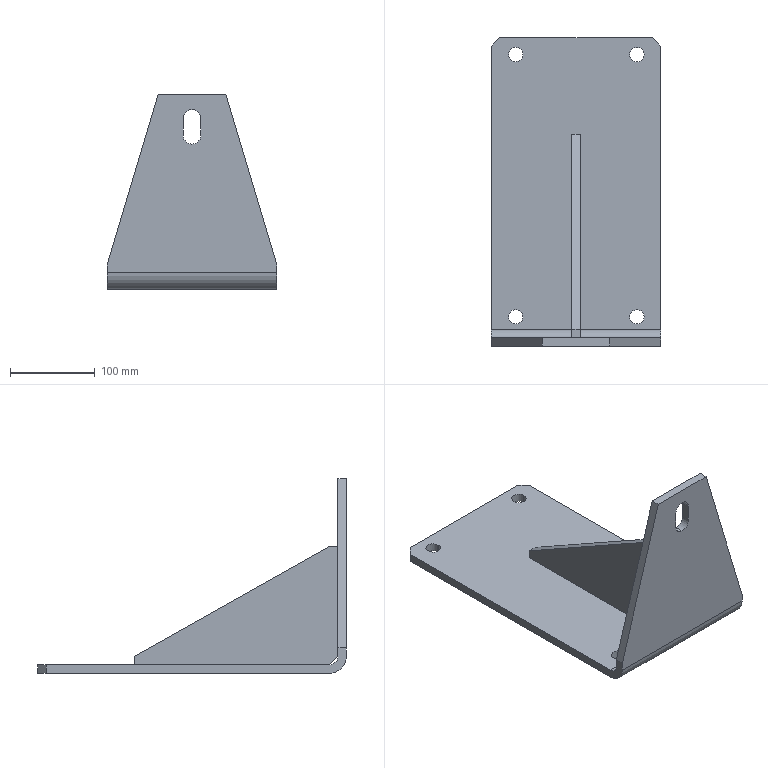Part | SolidWorks | features Chamfer 1, MBimport 1 | 1 solid | 33 faces | box 200 x 365 x 230 mm | volume 1205759 mm3 | plane 20 | cylinder 13 | commonest cylinder face diameters 17 x8 21 x3 20 x1 40 x1
STEP:
#1=CARTESIAN_POINT('',(183.597,184.249,10.));
#2=VERTEX_POINT('',#1);
#3=CARTESIAN_POINT('',(193.597,184.249,10.));
#4=VERTEX_POINT('',#3);
#5=CARTESIAN_POINT('',(183.597,184.249,10.));
#6=DIRECTION('',(1.,0.,0.));
#7=VECTOR('',#6,1000.);
#8=LINE('',#5,#7);
#9=EDGE_CURVE('',#2,#4,#8,.T.);
#10=ORIENTED_EDGE('',*,*,#9,.F.);
#11=CARTESIAN_POINT('',(88.597,184.249,10.));
#12=VERTEX_POINT('',#11);
#13=CARTESIAN_POINT('',(288.597,184.249,10.));
#14=DIRECTION('',(1.,0.,0.));
#15=VECTOR('',#14,1000.);
#16=LINE('',#13,#15);
#17=EDGE_CURVE('',#12,#2,#16,.T.);
#18=ORIENTED_EDGE('',*,*,#17,.F.);
#19=CARTESIAN_POINT('',(88.597,174.249,20.));
#20=VERTEX_POINT('',#19);
#21=CARTESIAN_POINT('',(88.597,184.249,20.));
#22=DIRECTION('',(1.,0.,0.));
#23=DIRECTION('',(0.,1.,0.));
#24=AXIS2_PLACEMENT_3D('',#21,#22,#23);
#25=CIRCLE('',#24,10.);
#26=EDGE_CURVE('',#20,#12,#25,.T.);
#27=ORIENTED_EDGE('',*,*,#26,.F.);
#28=CARTESIAN_POINT('',(183.597,174.249,20.));
#29=VERTEX_POINT('',#28);
#30=CARTESIAN_POINT('',(88.597,174.249,20.));
#31=DIRECTION('',(-1.,0.,0.));
#32=VECTOR('',#31,1000.);
#33=LINE('',#30,#32);
#34=EDGE_CURVE('',#29,#20,#33,.T.);
#35=ORIENTED_EDGE('',*,*,#34,.F.);
#36=CARTESIAN_POINT('',(193.597,174.249,20.));
#37=VERTEX_POINT('',#36);
#38=CARTESIAN_POINT('',(183.597,174.249,20.));
#39=DIRECTION('',(1.,0.,0.));
#40=VECTOR('',#39,1000.);
#41=LINE('',#38,#40);
#42=EDGE_CURVE('',#29,#37,#41,.T.);
#43=ORIENTED_EDGE('',*,*,#42,.T.);
#44=CARTESIAN_POINT('',(288.597,174.249,20.));
#45=VERTEX_POINT('',#44);
#46=CARTESIAN_POINT('',(88.597,174.249,20.));
#47=DIRECTION('',(-1.,0.,0.));
#48=VECTOR('',#47,1000.);
#49=LINE('',#46,#48);
#50=EDGE_CURVE('',#45,#37,#49,.T.);
#51=ORIENTED_EDGE('',*,*,#50,.F.);
#52=CARTESIAN_POINT('',(288.597,184.249,10.));
#53=VERTEX_POINT('',#52);
#54=CARTESIAN_POINT('',(288.597,184.249,20.));
#55=DIRECTION('',(-1.,0.,0.));
#56=DIRECTION('',(0.,-1.,0.));
#57=AXIS2_PLACEMENT_3D('',#54,#55,#56);
#58=CIRCLE('',#57,10.);
#59=EDGE_CURVE('',#53,#45,#58,.T.);
#60=ORIENTED_EDGE('',*,*,#59,.F.);
#61=CARTESIAN_POINT('',(288.597,184.249,10.));
#62=DIRECTION('',(1.,0.,0.));
#63=VECTOR('',#62,1000.);
#64=LINE('',#61,#63);
#65=EDGE_CURVE('',#4,#53,#64,.T.);
#66=ORIENTED_EDGE('',*,*,#65,.F.);
#67=EDGE_LOOP('',(#10,#18,#27,#35,#43,#51,#60,#66));
#68=FACE_OUTER_BOUND('',#67,.T.);
#69=CARTESIAN_POINT('',(0.,184.249,20.));
#70=DIRECTION('',(1.,0.,0.));
#71=DIRECTION('',(0.,0.,-1.));
#72=AXIS2_PLACEMENT_3D('',#69,#70,#71);
#73=CYLINDRICAL_SURFACE('',#72,10.);
#74=ADVANCED_FACE('',(#68),#73,.F.);
#75=CARTESIAN_POINT('',(88.597,184.249,0.));
#76=VERTEX_POINT('',#75);
#77=CARTESIAN_POINT('',(88.597,164.249,20.));
#78=VERTEX_POINT('',#77);
#79=CARTESIAN_POINT('',(88.597,184.249,20.));
#80=DIRECTION('',(-1.,0.,0.));
#81=DIRECTION('',(0.,1.,0.));
#82=AXIS2_PLACEMENT_3D('',#79,#80,#81);
#83=CIRCLE('',#82,20.);
#84=EDGE_CURVE('',#76,#78,#83,.T.);
#85=ORIENTED_EDGE('',*,*,#84,.F.);
#86=CARTESIAN_POINT('',(288.597,184.249,0.));
#87=VERTEX_POINT('',#86);
#88=CARTESIAN_POINT('',(88.597,184.249,0.));
#89=DIRECTION('',(-1.,0.,0.));
#90=VECTOR('',#89,1000.);
#91=LINE('',#88,#90);
#92=EDGE_CURVE('',#87,#76,#91,.T.);
#93=ORIENTED_EDGE('',*,*,#92,.F.);
#94=CARTESIAN_POINT('',(288.597,164.249,20.));
#95=VERTEX_POINT('',#94);
#96=CARTESIAN_POINT('',(288.597,184.249,20.));
#97=DIRECTION('',(1.,0.,0.));
#98=DIRECTION('',(0.,-1.,0.));
#99=AXIS2_PLACEMENT_3D('',#96,#97,#98);
#100=CIRCLE('',#99,20.);
#101=EDGE_CURVE('',#95,#87,#100,.T.);
#102=ORIENTED_EDGE('',*,*,#101,.F.);
#103=CARTESIAN_POINT('',(288.597,164.249,20.));
#104=DIRECTION('',(1.,0.,0.));
#105=VECTOR('',#104,1000.);
#106=LINE('',#103,#105);
#107=EDGE_CURVE('',#78,#95,#106,.T.);
#108=ORIENTED_EDGE('',*,*,#107,.F.);
#109=EDGE_LOOP('',(#85,#93,#102,#108));
#110=FACE_OUTER_BOUND('',#109,.T.);
#111=CARTESIAN_POINT('',(288.597,184.249,20.));
#112=DIRECTION('',(-1.,0.,0.));
#113=DIRECTION('',(0.,0.,1.));
#114=AXIS2_PLACEMENT_3D('',#111,#112,#113);
#115=CYLINDRICAL_SURFACE('',#114,20.);
#116=ADVANCED_FACE('',(#110),#115,.T.);
#117=CARTESIAN_POINT('',(193.597,414.753,10.));
#118=VERTEX_POINT('',#117);
#119=CARTESIAN_POINT('',(193.597,414.753,10.));
#120=DIRECTION('',(0.,-1.,0.));
#121=VECTOR('',#120,1000.);
#122=LINE('',#119,#121);
#123=EDGE_CURVE('',#118,#4,#122,.T.);
#124=ORIENTED_EDGE('',*,*,#123,.F.);
#125=CARTESIAN_POINT('',(193.597,414.753,20.));
#126=VERTEX_POINT('',#125);
#127=CARTESIAN_POINT('',(193.597,414.753,10.));
#128=DIRECTION('',(0.,0.,-1.));
#129=VECTOR('',#128,1000.);
#130=LINE('',#127,#129);
#131=EDGE_CURVE('',#126,#118,#130,.T.);
#132=ORIENTED_EDGE('',*,*,#131,.F.);
#133=CARTESIAN_POINT('',(193.597,184.249,150.));
#134=VERTEX_POINT('',#133);
#135=CARTESIAN_POINT('',(193.597,414.753,20.));
#136=DIRECTION('',(0.,0.871,-0.4912));
#137=VECTOR('',#136,1000.);
#138=LINE('',#135,#137);
#139=EDGE_CURVE('',#134,#126,#138,.T.);
#140=ORIENTED_EDGE('',*,*,#139,.F.);
#141=CARTESIAN_POINT('',(193.597,174.249,150.));
#142=VERTEX_POINT('',#141);
#143=CARTESIAN_POINT('',(193.597,184.249,150.));
#144=DIRECTION('',(0.,1.,0.));
#145=VECTOR('',#144,1000.);
#146=LINE('',#143,#145);
#147=EDGE_CURVE('',#142,#134,#146,.T.);
#148=ORIENTED_EDGE('',*,*,#147,.F.);
#149=CARTESIAN_POINT('',(193.597,174.249,20.));
#150=DIRECTION('',(0.,0.,1.));
#151=VECTOR('',#150,1000.);
#152=LINE('',#149,#151);
#153=EDGE_CURVE('',#37,#142,#152,.T.);
#154=ORIENTED_EDGE('',*,*,#153,.F.);
#155=CARTESIAN_POINT('',(193.597,184.249,10.));
#156=DIRECTION('',(0.,-0.7071,0.7071));
#157=VECTOR('',#156,1000.);
#158=LINE('',#155,#157);
#159=EDGE_CURVE('',#4,#37,#158,.T.);
#160=ORIENTED_EDGE('',*,*,#159,.F.);
#161=EDGE_LOOP('',(#124,#132,#140,#148,#154,#160));
#162=FACE_OUTER_BOUND('',#161,.T.);
#163=CARTESIAN_POINT('',(193.597,0.,0.));
#164=DIRECTION('',(-1.,0.,0.));
#165=DIRECTION('',(0.,1.,0.));
#166=AXIS2_PLACEMENT_3D('',#163,#164,#165);
#167=PLANE('',#166);
#168=ADVANCED_FACE('',(#162),#167,.F.);
#169=CARTESIAN_POINT('',(183.597,414.753,10.));
#170=VERTEX_POINT('',#169);
#171=CARTESIAN_POINT('',(183.597,414.753,10.));
#172=DIRECTION('',(0.,-1.,0.));
#173=VECTOR('',#172,1000.);
#174=LINE('',#171,#173);
#175=EDGE_CURVE('',#170,#2,#174,.T.);
#176=ORIENTED_EDGE('',*,*,#175,.T.);
#177=CARTESIAN_POINT('',(183.597,184.249,10.));
#178=DIRECTION('',(0.,-0.7071,0.7071));
#179=VECTOR('',#178,1000.);
#180=LINE('',#177,#179);
#181=EDGE_CURVE('',#2,#29,#180,.T.);
#182=ORIENTED_EDGE('',*,*,#181,.T.);
#183=CARTESIAN_POINT('',(183.597,174.249,150.));
#184=VERTEX_POINT('',#183);
#185=CARTESIAN_POINT('',(183.597,174.249,20.));
#186=DIRECTION('',(0.,0.,1.));
#187=VECTOR('',#186,1000.);
#188=LINE('',#185,#187);
#189=EDGE_CURVE('',#29,#184,#188,.T.);
#190=ORIENTED_EDGE('',*,*,#189,.T.);
#191=CARTESIAN_POINT('',(183.597,184.249,150.));
#192=VERTEX_POINT('',#191);
#193=CARTESIAN_POINT('',(183.597,184.249,150.));
#194=DIRECTION('',(0.,1.,0.));
#195=VECTOR('',#194,1000.);
#196=LINE('',#193,#195);
#197=EDGE_CURVE('',#184,#192,#196,.T.);
#198=ORIENTED_EDGE('',*,*,#197,.T.);
#199=CARTESIAN_POINT('',(183.597,414.753,20.));
#200=VERTEX_POINT('',#199);
#201=CARTESIAN_POINT('',(183.597,414.753,20.));
#202=DIRECTION('',(0.,0.871,-0.4912));
#203=VECTOR('',#202,1000.);
#204=LINE('',#201,#203);
#205=EDGE_CURVE('',#192,#200,#204,.T.);
#206=ORIENTED_EDGE('',*,*,#205,.T.);
#207=CARTESIAN_POINT('',(183.597,414.753,10.));
#208=DIRECTION('',(0.,0.,-1.));
#209=VECTOR('',#208,1000.);
#210=LINE('',#207,#209);
#211=EDGE_CURVE('',#200,#170,#210,.T.);
#212=ORIENTED_EDGE('',*,*,#211,.T.);
#213=EDGE_LOOP('',(#176,#182,#190,#198,#206,#212));
#214=FACE_OUTER_BOUND('',#213,.T.);
#215=CARTESIAN_POINT('',(183.597,0.,0.));
#216=DIRECTION('',(-1.,0.,0.));
#217=DIRECTION('',(0.,1.,0.));
#218=AXIS2_PLACEMENT_3D('',#215,#216,#217);
#219=PLANE('',#218);
#220=ADVANCED_FACE('',(#214),#219,.T.);
#221=ORIENTED_EDGE('',*,*,#131,.T.);
#222=CARTESIAN_POINT('',(183.597,414.753,10.));
#223=DIRECTION('',(1.,0.,0.));
#224=VECTOR('',#223,1000.);
#225=LINE('',#222,#224);
#226=EDGE_CURVE('',#170,#118,#225,.T.);
#227=ORIENTED_EDGE('',*,*,#226,.F.);
#228=ORIENTED_EDGE('',*,*,#211,.F.);
#229=CARTESIAN_POINT('',(183.597,414.753,20.));
#230=DIRECTION('',(1.,0.,0.));
#231=VECTOR('',#230,1000.);
#232=LINE('',#229,#231);
#233=EDGE_CURVE('',#200,#126,#232,.T.);
#234=ORIENTED_EDGE('',*,*,#233,.T.);
#235=EDGE_LOOP('',(#221,#227,#228,#234));
#236=FACE_OUTER_BOUND('',#235,.T.);
#237=CARTESIAN_POINT('',(183.597,414.753,10.));
#238=DIRECTION('',(0.,-1.,0.));
#239=DIRECTION('',(0.,0.,-1.));
#240=AXIS2_PLACEMENT_3D('',#237,#238,#239);
#241=PLANE('',#240);
#242=ADVANCED_FACE('',(#236),#241,.F.);
#243=ORIENTED_EDGE('',*,*,#139,.T.);
#244=ORIENTED_EDGE('',*,*,#233,.F.);
#245=ORIENTED_EDGE('',*,*,#205,.F.);
#246=CARTESIAN_POINT('',(183.597,184.249,150.));
#247=DIRECTION('',(1.,0.,0.));
#248=VECTOR('',#247,1000.);
#249=LINE('',#246,#248);
#250=EDGE_CURVE('',#192,#134,#249,.T.);
#251=ORIENTED_EDGE('',*,*,#250,.T.);
#252=EDGE_LOOP('',(#243,#244,#245,#251));
#253=FACE_OUTER_BOUND('',#252,.T.);
#254=CARTESIAN_POINT('',(183.597,414.753,20.));
#255=DIRECTION('',(0.,-0.4912,-0.871));
#256=DIRECTION('',(0.,-0.871,0.4912));
#257=AXIS2_PLACEMENT_3D('',#254,#255,#256);
#258=PLANE('',#257);
#259=ADVANCED_FACE('',(#253),#258,.F.);
#260=ORIENTED_EDGE('',*,*,#147,.T.);
#261=ORIENTED_EDGE('',*,*,#250,.F.);
#262=ORIENTED_EDGE('',*,*,#197,.F.);
#263=CARTESIAN_POINT('',(183.597,174.249,150.));
#264=DIRECTION('',(1.,0.,0.));
#265=VECTOR('',#264,1000.);
#266=LINE('',#263,#265);
#267=EDGE_CURVE('',#184,#142,#266,.T.);
#268=ORIENTED_EDGE('',*,*,#267,.T.);
#269=EDGE_LOOP('',(#260,#261,#262,#268));
#270=FACE_OUTER_BOUND('',#269,.T.);
#271=CARTESIAN_POINT('',(183.597,184.249,150.));
#272=DIRECTION('',(0.,0.,-1.));
#273=DIRECTION('',(0.,-1.,0.));
#274=AXIS2_PLACEMENT_3D('',#271,#272,#273);
#275=PLANE('',#274);
#276=ADVANCED_FACE('',(#270),#275,.F.);
#277=ORIENTED_EDGE('',*,*,#159,.T.);
#278=ORIENTED_EDGE('',*,*,#42,.F.);
#279=ORIENTED_EDGE('',*,*,#181,.F.);
#280=ORIENTED_EDGE('',*,*,#9,.T.);
#281=EDGE_LOOP('',(#277,#278,#279,#280));
#282=FACE_OUTER_BOUND('',#281,.T.);
#283=CARTESIAN_POINT('',(183.597,184.249,10.));
#284=DIRECTION('',(0.,0.7071,0.7071));
#285=DIRECTION('',(1.,0.,0.));
#286=AXIS2_PLACEMENT_3D('',#283,#284,#285);
#287=PLANE('',#286);
#288=ADVANCED_FACE('',(#282),#287,.F.);
#289=CARTESIAN_POINT('',(178.097,164.249,202.));
#290=VERTEX_POINT('',#289);
#291=CARTESIAN_POINT('',(178.097,164.249,182.));
#292=VERTEX_POINT('',#291);
#293=CARTESIAN_POINT('',(178.097,164.249,0.));
#294=DIRECTION('',(0.,0.,-1.));
#295=VECTOR('',#294,1000.);
#296=LINE('',#293,#295);
#297=EDGE_CURVE('',#290,#292,#296,.T.);
#298=ORIENTED_EDGE('',*,*,#297,.T.);
#299=CARTESIAN_POINT('',(178.097,174.249,182.));
#300=VERTEX_POINT('',#299);
#301=CARTESIAN_POINT('',(178.097,174.249,182.));
#302=DIRECTION('',(0.,-1.,0.));
#303=VECTOR('',#302,1000.);
#304=LINE('',#301,#303);
#305=EDGE_CURVE('',#300,#292,#304,.T.);
#306=ORIENTED_EDGE('',*,*,#305,.F.);
#307=CARTESIAN_POINT('',(178.097,174.249,202.));
#308=VERTEX_POINT('',#307);
#309=CARTESIAN_POINT('',(178.097,174.249,0.));
#310=DIRECTION('',(0.,0.,-1.));
#311=VECTOR('',#310,1000.);
#312=LINE('',#309,#311);
#313=EDGE_CURVE('',#308,#300,#312,.T.);
#314=ORIENTED_EDGE('',*,*,#313,.F.);
#315=CARTESIAN_POINT('',(178.097,174.249,202.));
#316=DIRECTION('',(0.,-1.,0.));
#317=VECTOR('',#316,1000.);
#318=LINE('',#315,#317);
#319=EDGE_CURVE('',#308,#290,#318,.T.);
#320=ORIENTED_EDGE('',*,*,#319,.T.);
#321=EDGE_LOOP('',(#298,#306,#314,#320));
#322=FACE_OUTER_BOUND('',#321,.T.);
#323=CARTESIAN_POINT('',(178.097,174.249,0.));
#324=DIRECTION('',(-1.,0.,0.));
#325=DIRECTION('',(0.,0.,1.));
#326=AXIS2_PLACEMENT_3D('',#323,#324,#325);
#327=PLANE('',#326);
#328=ADVANCED_FACE('',(#322),#327,.F.);
#329=CARTESIAN_POINT('',(148.597,164.249,230.));
#330=VERTEX_POINT('',#329);
#331=CARTESIAN_POINT('',(228.597,164.249,230.));
#332=VERTEX_POINT('',#331);
#333=CARTESIAN_POINT('',(0.,164.249,230.));
#334=DIRECTION('',(1.,0.,0.));
#335=VECTOR('',#334,1000.);
#336=LINE('',#333,#335);
#337=EDGE_CURVE('',#330,#332,#336,.T.);
#338=ORIENTED_EDGE('',*,*,#337,.T.);
#339=CARTESIAN_POINT('',(228.597,174.249,230.));
#340=VERTEX_POINT('',#339);
#341=CARTESIAN_POINT('',(228.597,174.249,230.));
#342=DIRECTION('',(0.,-1.,0.));
#343=VECTOR('',#342,1000.);
#344=LINE('',#341,#343);
#345=EDGE_CURVE('',#340,#332,#344,.T.);
#346=ORIENTED_EDGE('',*,*,#345,.F.);
#347=CARTESIAN_POINT('',(148.597,174.249,230.));
#348=VERTEX_POINT('',#347);
#349=CARTESIAN_POINT('',(0.,174.249,230.));
#350=DIRECTION('',(1.,0.,0.));
#351=VECTOR('',#350,1000.);
#352=LINE('',#349,#351);
#353=EDGE_CURVE('',#348,#340,#352,.T.);
#354=ORIENTED_EDGE('',*,*,#353,.F.);
#355=CARTESIAN_POINT('',(148.597,174.249,230.));
#356=DIRECTION('',(0.,-1.,0.));
#357=VECTOR('',#356,1000.);
#358=LINE('',#355,#357);
#359=EDGE_CURVE('',#348,#330,#358,.T.);
#360=ORIENTED_EDGE('',*,*,#359,.T.);
#361=EDGE_LOOP('',(#338,#346,#354,#360));
#362=FACE_OUTER_BOUND('',#361,.T.);
#363=CARTESIAN_POINT('',(0.,174.249,230.));
#364=DIRECTION('',(0.,0.,-1.));
#365=DIRECTION('',(0.,-1.,0.));
#366=AXIS2_PLACEMENT_3D('',#363,#364,#365);
#367=PLANE('',#366);
#368=ADVANCED_FACE('',(#362),#367,.F.);
#369=CARTESIAN_POINT('',(88.597,164.249,30.));
#370=VERTEX_POINT('',#369);
#371=CARTESIAN_POINT('',(73.025,164.249,-21.908));
#372=DIRECTION('',(0.2873,0.,0.9578));
#373=VECTOR('',#372,1000.);
#374=LINE('',#371,#373);
#375=EDGE_CURVE('',#370,#330,#374,.T.);
#376=ORIENTED_EDGE('',*,*,#375,.T.);
#377=ORIENTED_EDGE('',*,*,#359,.F.);
#378=CARTESIAN_POINT('',(88.597,174.249,30.));
#379=VERTEX_POINT('',#378);
#380=CARTESIAN_POINT('',(73.025,174.249,-21.908));
#381=DIRECTION('',(0.2873,0.,0.9578));
#382=VECTOR('',#381,1000.);
#383=LINE('',#380,#382);
#384=EDGE_CURVE('',#379,#348,#383,.T.);
#385=ORIENTED_EDGE('',*,*,#384,.F.);
#386=CARTESIAN_POINT('',(88.597,174.249,30.));
#387=DIRECTION('',(0.,-1.,0.));
#388=VECTOR('',#387,1000.);
#389=LINE('',#386,#388);
#390=EDGE_CURVE('',#379,#370,#389,.T.);
#391=ORIENTED_EDGE('',*,*,#390,.T.);
#392=EDGE_LOOP('',(#376,#377,#385,#391));
#393=FACE_OUTER_BOUND('',#392,.T.);
#394=CARTESIAN_POINT('',(73.025,174.249,-21.908));
#395=DIRECTION('',(0.9578,0.,-0.2873));
#396=DIRECTION('',(0.,-1.,0.));
#397=AXIS2_PLACEMENT_3D('',#394,#395,#396);
#398=PLANE('',#397);
#399=ADVANCED_FACE('',(#393),#398,.F.);
#400=CARTESIAN_POINT('',(288.597,164.249,30.));
#401=VERTEX_POINT('',#400);
#402=CARTESIAN_POINT('',(273.025,164.249,81.908));
#403=DIRECTION('',(0.2873,0.,-0.9578));
#404=VECTOR('',#403,1000.);
#405=LINE('',#402,#404);
#406=EDGE_CURVE('',#332,#401,#405,.T.);
#407=ORIENTED_EDGE('',*,*,#406,.T.);
#408=CARTESIAN_POINT('',(288.597,174.249,30.));
#409=VERTEX_POINT('',#408);
#410=CARTESIAN_POINT('',(288.597,174.249,30.));
#411=DIRECTION('',(0.,-1.,0.));
#412=VECTOR('',#411,1000.);
#413=LINE('',#410,#412);
#414=EDGE_CURVE('',#409,#401,#413,.T.);
#415=ORIENTED_EDGE('',*,*,#414,.F.);
#416=CARTESIAN_POINT('',(273.025,174.249,81.908));
#417=DIRECTION('',(0.2873,0.,-0.9578));
#418=VECTOR('',#417,1000.);
#419=LINE('',#416,#418);
#420=EDGE_CURVE('',#340,#409,#419,.T.);
#421=ORIENTED_EDGE('',*,*,#420,.F.);
#422=ORIENTED_EDGE('',*,*,#345,.T.);
#423=EDGE_LOOP('',(#407,#415,#421,#422));
#424=FACE_OUTER_BOUND('',#423,.T.);
#425=CARTESIAN_POINT('',(273.025,174.249,81.908));
#426=DIRECTION('',(-0.9578,0.,-0.2873));
#427=DIRECTION('',(-0.2873,0.,0.9578));
#428=AXIS2_PLACEMENT_3D('',#425,#426,#427);
#429=PLANE('',#428);
#430=ADVANCED_FACE('',(#424),#429,.F.);
#431=CARTESIAN_POINT('',(199.097,164.249,202.));
#432=VERTEX_POINT('',#431);
#433=CARTESIAN_POINT('',(188.597,164.249,202.));
#434=DIRECTION('',(0.,-1.,0.));
#435=DIRECTION('',(0.,0.,-1.));
#436=AXIS2_PLACEMENT_3D('',#433,#434,#435);
#437=CIRCLE('',#436,10.5);
#438=EDGE_CURVE('',#432,#290,#437,.T.);
#439=ORIENTED_EDGE('',*,*,#438,.T.);
#440=ORIENTED_EDGE('',*,*,#319,.F.);
#441=CARTESIAN_POINT('',(199.097,174.249,202.));
#442=VERTEX_POINT('',#441);
#443=CARTESIAN_POINT('',(188.597,174.249,202.));
#444=DIRECTION('',(0.,-1.,0.));
#445=DIRECTION('',(0.,0.,-1.));
#446=AXIS2_PLACEMENT_3D('',#443,#444,#445);
#447=CIRCLE('',#446,10.5);
#448=EDGE_CURVE('',#442,#308,#447,.T.);
#449=ORIENTED_EDGE('',*,*,#448,.F.);
#450=CARTESIAN_POINT('',(199.097,174.249,202.));
#451=DIRECTION('',(0.,-1.,0.));
#452=VECTOR('',#451,1000.);
#453=LINE('',#450,#452);
#454=EDGE_CURVE('',#442,#432,#453,.T.);
#455=ORIENTED_EDGE('',*,*,#454,.T.);
#456=EDGE_LOOP('',(#439,#440,#449,#455));
#457=FACE_OUTER_BOUND('',#456,.T.);
#458=CARTESIAN_POINT('',(188.597,174.249,202.));
#459=DIRECTION('',(0.,-1.,0.));
#460=DIRECTION('',(0.,0.,-1.));
#461=AXIS2_PLACEMENT_3D('',#458,#459,#460);
#462=CYLINDRICAL_SURFACE('',#461,10.5);
#463=ADVANCED_FACE('',(#457),#462,.F.);
#464=CARTESIAN_POINT('',(199.097,164.249,182.));
#465=VERTEX_POINT('',#464);
#466=CARTESIAN_POINT('',(199.097,164.249,0.));
#467=DIRECTION('',(0.,0.,-1.));
#468=VECTOR('',#467,1000.);
#469=LINE('',#466,#468);
#470=EDGE_CURVE('',#432,#465,#469,.T.);
#471=ORIENTED_EDGE('',*,*,#470,.F.);
#472=ORIENTED_EDGE('',*,*,#454,.F.);
#473=CARTESIAN_POINT('',(199.097,174.249,182.));
#474=VERTEX_POINT('',#473);
#475=CARTESIAN_POINT('',(199.097,174.249,0.));
#476=DIRECTION('',(0.,0.,-1.));
#477=VECTOR('',#476,1000.);
#478=LINE('',#475,#477);
#479=EDGE_CURVE('',#442,#474,#478,.T.);
#480=ORIENTED_EDGE('',*,*,#479,.T.);
#481=CARTESIAN_POINT('',(199.097,174.249,182.));
#482=DIRECTION('',(0.,-1.,0.));
#483=VECTOR('',#482,1000.);
#484=LINE('',#481,#483);
#485=EDGE_CURVE('',#474,#465,#484,.T.);
#486=ORIENTED_EDGE('',*,*,#485,.T.);
#487=EDGE_LOOP('',(#471,#472,#480,#486));
#488=FACE_OUTER_BOUND('',#487,.T.);
#489=CARTESIAN_POINT('',(199.097,174.249,0.));
#490=DIRECTION('',(-1.,0.,0.));
#491=DIRECTION('',(0.,0.,1.));
#492=AXIS2_PLACEMENT_3D('',#489,#490,#491);
#493=PLANE('',#492);
#494=ADVANCED_FACE('',(#488),#493,.T.);
#495=CARTESIAN_POINT('',(188.597,174.249,171.5));
#496=VERTEX_POINT('',#495);
#497=CARTESIAN_POINT('',(188.597,164.249,171.5));
#498=VERTEX_POINT('',#497);
#499=CARTESIAN_POINT('',(188.597,174.249,171.5));
#500=DIRECTION('',(0.,-1.,0.));
#501=VECTOR('',#500,1000.);
#502=LINE('',#499,#501);
#503=EDGE_CURVE('',#496,#498,#502,.T.);
#504=ORIENTED_EDGE('',*,*,#503,.F.);
#505=CARTESIAN_POINT('',(188.597,174.249,182.));
#506=DIRECTION('',(0.,-1.,0.));
#507=DIRECTION('',(0.,0.,-1.));
#508=AXIS2_PLACEMENT_3D('',#505,#506,#507);
#509=CIRCLE('',#508,10.5);
#510=EDGE_CURVE('',#300,#496,#509,.T.);
#511=ORIENTED_EDGE('',*,*,#510,.F.);
#512=ORIENTED_EDGE('',*,*,#305,.T.);
#513=CARTESIAN_POINT('',(188.597,164.249,182.));
#514=DIRECTION('',(0.,-1.,0.));
#515=DIRECTION('',(0.,0.,-1.));
#516=AXIS2_PLACEMENT_3D('',#513,#514,#515);
#517=CIRCLE('',#516,10.5);
#518=EDGE_CURVE('',#292,#498,#517,.T.);
#519=ORIENTED_EDGE('',*,*,#518,.T.);
#520=EDGE_LOOP('',(#504,#511,#512,#519));
#521=FACE_OUTER_BOUND('',#520,.T.);
#522=CARTESIAN_POINT('',(188.597,174.249,182.));
#523=DIRECTION('',(0.,-1.,0.));
#524=DIRECTION('',(0.,0.,-1.));
#525=AXIS2_PLACEMENT_3D('',#522,#523,#524);
#526=CYLINDRICAL_SURFACE('',#525,10.5);
#527=ADVANCED_FACE('',(#521),#526,.F.);
#528=ORIENTED_EDGE('',*,*,#510,.T.);
#529=CARTESIAN_POINT('',(188.597,174.249,182.));
#530=DIRECTION('',(0.,-1.,0.));
#531=DIRECTION('',(0.,0.,-1.));
#532=AXIS2_PLACEMENT_3D('',#529,#530,#531);
#533=CIRCLE('',#532,10.5);
#534=EDGE_CURVE('',#496,#474,#533,.T.);
#535=ORIENTED_EDGE('',*,*,#534,.T.);
#536=ORIENTED_EDGE('',*,*,#479,.F.);
#537=ORIENTED_EDGE('',*,*,#448,.T.);
#538=ORIENTED_EDGE('',*,*,#313,.T.);
#539=EDGE_LOOP('',(#528,#535,#536,#537,#538));
#540=FACE_BOUND('',#539,.T.);
#541=CARTESIAN_POINT('',(288.597,174.249,0.));
#542=DIRECTION('',(0.,0.,-1.));
#543=VECTOR('',#542,1000.);
#544=LINE('',#541,#543);
#545=EDGE_CURVE('',#409,#45,#544,.T.);
#546=ORIENTED_EDGE('',*,*,#545,.T.);
#547=ORIENTED_EDGE('',*,*,#50,.T.);
#548=ORIENTED_EDGE('',*,*,#153,.T.);
#549=ORIENTED_EDGE('',*,*,#267,.F.);
#550=ORIENTED_EDGE('',*,*,#189,.F.);
#551=ORIENTED_EDGE('',*,*,#34,.T.);
#552=CARTESIAN_POINT('',(88.597,174.249,0.));
#553=DIRECTION('',(0.,0.,1.));
#554=VECTOR('',#553,1000.);
#555=LINE('',#552,#554);
#556=EDGE_CURVE('',#20,#379,#555,.T.);
#557=ORIENTED_EDGE('',*,*,#556,.T.);
#558=ORIENTED_EDGE('',*,*,#384,.T.);
#559=ORIENTED_EDGE('',*,*,#353,.T.);
#560=ORIENTED_EDGE('',*,*,#420,.T.);
#561=EDGE_LOOP('',(#546,#547,#548,#549,#550,#551,#557,#558,#559,#560));
#562=FACE_OUTER_BOUND('',#561,.T.);
#563=CARTESIAN_POINT('',(0.,174.249,0.));
#564=DIRECTION('',(0.,-1.,0.));
#565=DIRECTION('',(0.,0.,-1.));
#566=AXIS2_PLACEMENT_3D('',#563,#564,#565);
#567=PLANE('',#566);
#568=ADVANCED_FACE('',(#540,#562),#567,.F.);
#569=CARTESIAN_POINT('',(125.829,199.249,10.));
#570=VERTEX_POINT('',#569);
#571=CARTESIAN_POINT('',(125.829,199.249,0.));
#572=VERTEX_POINT('',#571);
#573=CARTESIAN_POINT('',(125.829,199.249,10.));
#574=DIRECTION('',(0.,0.,-1.));
#575=VECTOR('',#574,1000.);
#576=LINE('',#573,#575);
#577=EDGE_CURVE('',#570,#572,#576,.T.);
#578=ORIENTED_EDGE('',*,*,#577,.F.);
#579=CARTESIAN_POINT('',(108.829,199.249,10.));
#580=VERTEX_POINT('',#579);
#581=CARTESIAN_POINT('',(117.329,199.249,10.));
#582=DIRECTION('',(0.,0.,1.));
#583=DIRECTION('',(1.,0.,0.));
#584=AXIS2_PLACEMENT_3D('',#581,#582,#583);
#585=CIRCLE('',#584,8.5);
#586=EDGE_CURVE('',#570,#580,#585,.T.);
#587=ORIENTED_EDGE('',*,*,#586,.T.);
#588=CARTESIAN_POINT('',(108.829,199.249,0.));
#589=VERTEX_POINT('',#588);
#590=CARTESIAN_POINT('',(108.829,199.249,10.));
#591=DIRECTION('',(0.,0.,-1.));
#592=VECTOR('',#591,1000.);
#593=LINE('',#590,#592);
#594=EDGE_CURVE('',#580,#589,#593,.T.);
#595=ORIENTED_EDGE('',*,*,#594,.T.);
#596=CARTESIAN_POINT('',(117.329,199.249,0.));
#597=DIRECTION('',(0.,0.,1.));
#598=DIRECTION('',(1.,0.,0.));
#599=AXIS2_PLACEMENT_3D('',#596,#597,#598);
#600=CIRCLE('',#599,8.5);
#601=EDGE_CURVE('',#572,#589,#600,.T.);
#602=ORIENTED_EDGE('',*,*,#601,.F.);
#603=EDGE_LOOP('',(#578,#587,#595,#602));
#604=FACE_OUTER_BOUND('',#603,.T.);
#605=CARTESIAN_POINT('',(117.329,199.249,10.));
#606=DIRECTION('',(0.,0.,-1.));
#607=DIRECTION('',(-1.,0.,0.));
#608=AXIS2_PLACEMENT_3D('',#605,#606,#607);
#609=CYLINDRICAL_SURFACE('',#608,8.5);
#610=ADVANCED_FACE('',(#604),#609,.F.);
#611=CARTESIAN_POINT('',(269.135,199.249,10.));
#612=VERTEX_POINT('',#611);
#613=CARTESIAN_POINT('',(269.135,199.249,0.));
#614=VERTEX_POINT('',#613);
#615=CARTESIAN_POINT('',(269.135,199.249,10.));
#616=DIRECTION('',(0.,0.,-1.));
#617=VECTOR('',#616,1000.);
#618=LINE('',#615,#617);
#619=EDGE_CURVE('',#612,#614,#618,.T.);
#620=ORIENTED_EDGE('',*,*,#619,.F.);
#621=CARTESIAN_POINT('',(252.135,199.249,10.));
#622=VERTEX_POINT('',#621);
#623=CARTESIAN_POINT('',(260.635,199.249,10.));
#624=DIRECTION('',(0.,0.,1.));
#625=DIRECTION('',(1.,0.,0.));
#626=AXIS2_PLACEMENT_3D('',#623,#624,#625);
#627=CIRCLE('',#626,8.5);
#628=EDGE_CURVE('',#612,#622,#627,.T.);
#629=ORIENTED_EDGE('',*,*,#628,.T.);
#630=CARTESIAN_POINT('',(252.135,199.249,0.));
#631=VERTEX_POINT('',#630);
#632=CARTESIAN_POINT('',(252.135,199.249,10.));
#633=DIRECTION('',(0.,0.,-1.));
#634=VECTOR('',#633,1000.);
#635=LINE('',#632,#634);
#636=EDGE_CURVE('',#622,#631,#635,.T.);
#637=ORIENTED_EDGE('',*,*,#636,.T.);
#638=CARTESIAN_POINT('',(260.635,199.249,0.));
#639=DIRECTION('',(0.,0.,1.));
#640=DIRECTION('',(1.,0.,0.));
#641=AXIS2_PLACEMENT_3D('',#638,#639,#640);
#642=CIRCLE('',#641,8.5);
#643=EDGE_CURVE('',#614,#631,#642,.T.);
#644=ORIENTED_EDGE('',*,*,#643,.F.);
#645=EDGE_LOOP('',(#620,#629,#637,#644));
#646=FACE_OUTER_BOUND('',#645,.T.);
#647=CARTESIAN_POINT('',(260.635,199.249,10.));
#648=DIRECTION('',(0.,0.,-1.));
#649=DIRECTION('',(-1.,0.,0.));
#650=AXIS2_PLACEMENT_3D('',#647,#648,#649);
#651=CYLINDRICAL_SURFACE('',#650,8.5);
#652=ADVANCED_FACE('',(#646),#651,.F.);
#653=CARTESIAN_POINT('',(269.135,509.249,10.));
#654=VERTEX_POINT('',#653);
#655=CARTESIAN_POINT('',(269.135,509.249,0.));
#656=VERTEX_POINT('',#655);
#657=CARTESIAN_POINT('',(269.135,509.249,10.));
#658=DIRECTION('',(0.,0.,-1.));
#659=VECTOR('',#658,1000.);
#660=LINE('',#657,#659);
#661=EDGE_CURVE('',#654,#656,#660,.T.);
#662=ORIENTED_EDGE('',*,*,#661,.F.);
#663=CARTESIAN_POINT('',(252.135,509.249,10.));
#664=VERTEX_POINT('',#663);
#665=CARTESIAN_POINT('',(260.635,509.249,10.));
#666=DIRECTION('',(0.,0.,1.));
#667=DIRECTION('',(1.,0.,0.));
#668=AXIS2_PLACEMENT_3D('',#665,#666,#667);
#669=CIRCLE('',#668,8.5);
#670=EDGE_CURVE('',#654,#664,#669,.T.);
#671=ORIENTED_EDGE('',*,*,#670,.T.);
#672=CARTESIAN_POINT('',(252.135,509.249,0.));
#673=VERTEX_POINT('',#672);
#674=CARTESIAN_POINT('',(252.135,509.249,10.));
#675=DIRECTION('',(0.,0.,-1.));
#676=VECTOR('',#675,1000.);
#677=LINE('',#674,#676);
#678=EDGE_CURVE('',#664,#673,#677,.T.);
#679=ORIENTED_EDGE('',*,*,#678,.T.);
#680=CARTESIAN_POINT('',(260.635,509.249,0.));
#681=DIRECTION('',(0.,0.,1.));
#682=DIRECTION('',(1.,0.,0.));
#683=AXIS2_PLACEMENT_3D('',#680,#681,#682);
#684=CIRCLE('',#683,8.5);
#685=EDGE_CURVE('',#656,#673,#684,.T.);
#686=ORIENTED_EDGE('',*,*,#685,.F.);
#687=EDGE_LOOP('',(#662,#671,#679,#686));
#688=FACE_OUTER_BOUND('',#687,.T.);
#689=CARTESIAN_POINT('',(260.635,509.249,10.));
#690=DIRECTION('',(0.,0.,-1.));
#691=DIRECTION('',(-1.,0.,0.));
#692=AXIS2_PLACEMENT_3D('',#689,#690,#691);
#693=CYLINDRICAL_SURFACE('',#692,8.5);
#694=ADVANCED_FACE('',(#688),#693,.F.);
#695=CARTESIAN_POINT('',(125.829,509.249,10.));
#696=VERTEX_POINT('',#695);
#697=CARTESIAN_POINT('',(125.829,509.249,0.));
#698=VERTEX_POINT('',#697);
#699=CARTESIAN_POINT('',(125.829,509.249,10.));
#700=DIRECTION('',(0.,0.,-1.));
#701=VECTOR('',#700,1000.);
#702=LINE('',#699,#701);
#703=EDGE_CURVE('',#696,#698,#702,.T.);
#704=ORIENTED_EDGE('',*,*,#703,.F.);
#705=CARTESIAN_POINT('',(108.829,509.249,10.));
#706=VERTEX_POINT('',#705);
#707=CARTESIAN_POINT('',(117.329,509.249,10.));
#708=DIRECTION('',(0.,0.,1.));
#709=DIRECTION('',(1.,0.,0.));
#710=AXIS2_PLACEMENT_3D('',#707,#708,#709);
#711=CIRCLE('',#710,8.5);
#712=EDGE_CURVE('',#696,#706,#711,.T.);
#713=ORIENTED_EDGE('',*,*,#712,.T.);
#714=CARTESIAN_POINT('',(108.829,509.249,0.));
#715=VERTEX_POINT('',#714);
#716=CARTESIAN_POINT('',(108.829,509.249,10.));
#717=DIRECTION('',(0.,0.,-1.));
#718=VECTOR('',#717,1000.);
#719=LINE('',#716,#718);
#720=EDGE_CURVE('',#706,#715,#719,.T.);
#721=ORIENTED_EDGE('',*,*,#720,.T.);
#722=CARTESIAN_POINT('',(117.329,509.249,0.));
#723=DIRECTION('',(0.,0.,1.));
#724=DIRECTION('',(1.,0.,0.));
#725=AXIS2_PLACEMENT_3D('',#722,#723,#724);
#726=CIRCLE('',#725,8.5);
#727=EDGE_CURVE('',#698,#715,#726,.T.);
#728=ORIENTED_EDGE('',*,*,#727,.F.);
#729=EDGE_LOOP('',(#704,#713,#721,#728));
#730=FACE_OUTER_BOUND('',#729,.T.);
#731=CARTESIAN_POINT('',(117.329,509.249,10.));
#732=DIRECTION('',(0.,0.,-1.));
#733=DIRECTION('',(-1.,0.,0.));
#734=AXIS2_PLACEMENT_3D('',#731,#732,#733);
#735=CYLINDRICAL_SURFACE('',#734,8.5);
#736=ADVANCED_FACE('',(#730),#735,.F.);
#737=ORIENTED_EDGE('',*,*,#518,.F.);
#738=ORIENTED_EDGE('',*,*,#297,.F.);
#739=ORIENTED_EDGE('',*,*,#438,.F.);
#740=ORIENTED_EDGE('',*,*,#470,.T.);
#741=CARTESIAN_POINT('',(188.597,164.249,182.));
#742=DIRECTION('',(0.,-1.,0.));
#743=DIRECTION('',(0.,0.,-1.));
#744=AXIS2_PLACEMENT_3D('',#741,#742,#743);
#745=CIRCLE('',#744,10.5);
#746=EDGE_CURVE('',#498,#465,#745,.T.);
#747=ORIENTED_EDGE('',*,*,#746,.F.);
#748=EDGE_LOOP('',(#737,#738,#739,#740,#747));
#749=FACE_BOUND('',#748,.T.);
#750=CARTESIAN_POINT('',(88.597,164.249,10.));
#751=DIRECTION('',(0.,0.,-1.));
#752=VECTOR('',#751,1000.);
#753=LINE('',#750,#752);
#754=EDGE_CURVE('',#370,#78,#753,.T.);
#755=ORIENTED_EDGE('',*,*,#754,.T.);
#756=ORIENTED_EDGE('',*,*,#107,.T.);
#757=CARTESIAN_POINT('',(288.597,164.249,10.));
#758=DIRECTION('',(0.,0.,-1.));
#759=VECTOR('',#758,1000.);
#760=LINE('',#757,#759);
#761=EDGE_CURVE('',#401,#95,#760,.T.);
#762=ORIENTED_EDGE('',*,*,#761,.F.);
#763=ORIENTED_EDGE('',*,*,#406,.F.);
#764=ORIENTED_EDGE('',*,*,#337,.F.);
#765=ORIENTED_EDGE('',*,*,#375,.F.);
#766=EDGE_LOOP('',(#755,#756,#762,#763,#764,#765));
#767=FACE_OUTER_BOUND('',#766,.T.);
#768=CARTESIAN_POINT('',(288.597,164.249,10.));
#769=DIRECTION('',(0.,1.,0.));
#770=DIRECTION('',(1.,0.,0.));
#771=AXIS2_PLACEMENT_3D('',#768,#769,#770);
#772=PLANE('',#771);
#773=ADVANCED_FACE('',(#749,#767),#772,.F.);
#774=CARTESIAN_POINT('',(88.597,519.249,10.));
#775=VERTEX_POINT('',#774);
#776=CARTESIAN_POINT('',(88.597,529.249,10.));
#777=DIRECTION('',(0.,-1.,0.));
#778=VECTOR('',#777,1000.);
#779=LINE('',#776,#778);
#780=EDGE_CURVE('',#775,#12,#779,.T.);
#781=ORIENTED_EDGE('',*,*,#780,.F.);
#782=CARTESIAN_POINT('',(88.597,519.249,0.));
#783=VERTEX_POINT('',#782);
#784=CARTESIAN_POINT('',(88.597,519.249,10.));
#785=DIRECTION('',(0.,0.,-1.));
#786=VECTOR('',#785,1000.);
#787=LINE('',#784,#786);
#788=EDGE_CURVE('',#775,#783,#787,.T.);
#789=ORIENTED_EDGE('',*,*,#788,.T.);
#790=CARTESIAN_POINT('',(88.597,529.249,0.));
#791=DIRECTION('',(0.,-1.,0.));
#792=VECTOR('',#791,1000.);
#793=LINE('',#790,#792);
#794=EDGE_CURVE('',#783,#76,#793,.T.);
#795=ORIENTED_EDGE('',*,*,#794,.T.);
#796=ORIENTED_EDGE('',*,*,#84,.T.);
#797=ORIENTED_EDGE('',*,*,#754,.F.);
#798=ORIENTED_EDGE('',*,*,#390,.F.);
#799=ORIENTED_EDGE('',*,*,#556,.F.);
#800=ORIENTED_EDGE('',*,*,#26,.T.);
#801=EDGE_LOOP('',(#781,#789,#795,#796,#797,#798,#799,#800));
#802=FACE_OUTER_BOUND('',#801,.T.);
#803=CARTESIAN_POINT('',(88.597,529.249,10.));
#804=DIRECTION('',(1.,0.,0.));
#805=DIRECTION('',(0.,1.,0.));
#806=AXIS2_PLACEMENT_3D('',#803,#804,#805);
#807=PLANE('',#806);
#808=ADVANCED_FACE('',(#802),#807,.F.);
#809=CARTESIAN_POINT('',(278.597,529.249,0.));
#810=VERTEX_POINT('',#809);
#811=CARTESIAN_POINT('',(98.597,529.249,0.));
#812=VERTEX_POINT('',#811);
#813=CARTESIAN_POINT('',(288.597,529.249,0.));
#814=DIRECTION('',(-1.,0.,0.));
#815=VECTOR('',#814,1000.);
#816=LINE('',#813,#815);
#817=EDGE_CURVE('',#810,#812,#816,.T.);
#818=ORIENTED_EDGE('',*,*,#817,.T.);
#819=CARTESIAN_POINT('',(98.597,529.249,10.));
#820=VERTEX_POINT('',#819);
#821=CARTESIAN_POINT('',(98.597,529.249,10.));
#822=DIRECTION('',(0.,0.,1.));
#823=VECTOR('',#822,1000.);
#824=LINE('',#821,#823);
#825=EDGE_CURVE('',#812,#820,#824,.T.);
#826=ORIENTED_EDGE('',*,*,#825,.T.);
#827=CARTESIAN_POINT('',(278.597,529.249,10.));
#828=VERTEX_POINT('',#827);
#829=CARTESIAN_POINT('',(288.597,529.249,10.));
#830=DIRECTION('',(-1.,0.,0.));
#831=VECTOR('',#830,1000.);
#832=LINE('',#829,#831);
#833=EDGE_CURVE('',#828,#820,#832,.T.);
#834=ORIENTED_EDGE('',*,*,#833,.F.);
#835=CARTESIAN_POINT('',(278.597,529.249,10.));
#836=DIRECTION('',(0.,0.,-1.));
#837=VECTOR('',#836,1000.);
#838=LINE('',#835,#837);
#839=EDGE_CURVE('',#828,#810,#838,.T.);
#840=ORIENTED_EDGE('',*,*,#839,.T.);
#841=EDGE_LOOP('',(#818,#826,#834,#840));
#842=FACE_OUTER_BOUND('',#841,.T.);
#843=CARTESIAN_POINT('',(288.597,529.249,10.));
#844=DIRECTION('',(0.,-1.,0.));
#845=DIRECTION('',(0.,0.,-1.));
#846=AXIS2_PLACEMENT_3D('',#843,#844,#845);
#847=PLANE('',#846);
#848=ADVANCED_FACE('',(#842),#847,.F.);
#849=CARTESIAN_POINT('',(288.597,519.249,0.));
#850=VERTEX_POINT('',#849);
#851=CARTESIAN_POINT('',(288.597,529.249,0.));
#852=DIRECTION('',(0.,1.,0.));
#853=VECTOR('',#852,1000.);
#854=LINE('',#851,#853);
#855=EDGE_CURVE('',#87,#850,#854,.T.);
#856=ORIENTED_EDGE('',*,*,#855,.T.);
#857=CARTESIAN_POINT('',(288.597,519.249,10.));
#858=VERTEX_POINT('',#857);
#859=CARTESIAN_POINT('',(288.597,519.249,10.));
#860=DIRECTION('',(0.,0.,1.));
#861=VECTOR('',#860,1000.);
#862=LINE('',#859,#861);
#863=EDGE_CURVE('',#850,#858,#862,.T.);
#864=ORIENTED_EDGE('',*,*,#863,.T.);
#865=CARTESIAN_POINT('',(288.597,529.249,10.));
#866=DIRECTION('',(0.,1.,0.));
#867=VECTOR('',#866,1000.);
#868=LINE('',#865,#867);
#869=EDGE_CURVE('',#53,#858,#868,.T.);
#870=ORIENTED_EDGE('',*,*,#869,.F.);
#871=ORIENTED_EDGE('',*,*,#59,.T.);
#872=ORIENTED_EDGE('',*,*,#545,.F.);
#873=ORIENTED_EDGE('',*,*,#414,.T.);
#874=ORIENTED_EDGE('',*,*,#761,.T.);
#875=ORIENTED_EDGE('',*,*,#101,.T.);
#876=EDGE_LOOP('',(#856,#864,#870,#871,#872,#873,#874,#875));
#877=FACE_OUTER_BOUND('',#876,.T.);
#878=CARTESIAN_POINT('',(288.597,529.249,10.));
#879=DIRECTION('',(-1.,0.,0.));
#880=DIRECTION('',(0.,1.,0.));
#881=AXIS2_PLACEMENT_3D('',#878,#879,#880);
#882=PLANE('',#881);
#883=ADVANCED_FACE('',(#877),#882,.F.);
#884=CARTESIAN_POINT('',(117.329,199.249,0.));
#885=DIRECTION('',(0.,0.,1.));
#886=DIRECTION('',(1.,0.,0.));
#887=AXIS2_PLACEMENT_3D('',#884,#885,#886);
#888=CIRCLE('',#887,8.5);
#889=EDGE_CURVE('',#589,#572,#888,.T.);
#890=ORIENTED_EDGE('',*,*,#889,.T.);
#891=ORIENTED_EDGE('',*,*,#601,.T.);
#892=EDGE_LOOP('',(#890,#891));
#893=FACE_BOUND('',#892,.T.);
#894=CARTESIAN_POINT('',(260.635,509.249,0.));
#895=DIRECTION('',(0.,0.,1.));
#896=DIRECTION('',(1.,0.,0.));
#897=AXIS2_PLACEMENT_3D('',#894,#895,#896);
#898=CIRCLE('',#897,8.5);
#899=EDGE_CURVE('',#673,#656,#898,.T.);
#900=ORIENTED_EDGE('',*,*,#899,.T.);
#901=ORIENTED_EDGE('',*,*,#685,.T.);
#902=EDGE_LOOP('',(#900,#901));
#903=FACE_BOUND('',#902,.T.);
#904=CARTESIAN_POINT('',(117.329,509.249,0.));
#905=DIRECTION('',(0.,0.,1.));
#906=DIRECTION('',(1.,0.,0.));
#907=AXIS2_PLACEMENT_3D('',#904,#905,#906);
#908=CIRCLE('',#907,8.5);
#909=EDGE_CURVE('',#715,#698,#908,.T.);
#910=ORIENTED_EDGE('',*,*,#909,.T.);
#911=ORIENTED_EDGE('',*,*,#727,.T.);
#912=EDGE_LOOP('',(#910,#911));
#913=FACE_BOUND('',#912,.T.);
#914=CARTESIAN_POINT('',(260.635,199.249,0.));
#915=DIRECTION('',(0.,0.,1.));
#916=DIRECTION('',(1.,0.,0.));
#917=AXIS2_PLACEMENT_3D('',#914,#915,#916);
#918=CIRCLE('',#917,8.5);
#919=EDGE_CURVE('',#631,#614,#918,.T.);
#920=ORIENTED_EDGE('',*,*,#919,.T.);
#921=ORIENTED_EDGE('',*,*,#643,.T.);
#922=EDGE_LOOP('',(#920,#921));
#923=FACE_BOUND('',#922,.T.);
#924=ORIENTED_EDGE('',*,*,#794,.F.);
#925=CARTESIAN_POINT('',(-215.326,215.326,0.));
#926=DIRECTION('',(0.7071,0.7071,0.));
#927=VECTOR('',#926,1000.);
#928=LINE('',#925,#927);
#929=EDGE_CURVE('',#783,#812,#928,.T.);
#930=ORIENTED_EDGE('',*,*,#929,.T.);
#931=ORIENTED_EDGE('',*,*,#817,.F.);
#932=CARTESIAN_POINT('',(403.923,403.923,0.));
#933=DIRECTION('',(0.7071,-0.7071,0.));
#934=VECTOR('',#933,1000.);
#935=LINE('',#932,#934);
#936=EDGE_CURVE('',#810,#850,#935,.T.);
#937=ORIENTED_EDGE('',*,*,#936,.T.);
#938=ORIENTED_EDGE('',*,*,#855,.F.);
#939=ORIENTED_EDGE('',*,*,#92,.T.);
#940=EDGE_LOOP('',(#924,#930,#931,#937,#938,#939));
#941=FACE_OUTER_BOUND('',#940,.T.);
#942=CARTESIAN_POINT('',(0.,0.,0.));
#943=DIRECTION('',(0.,0.,-1.));
#944=DIRECTION('',(0.,-1.,0.));
#945=AXIS2_PLACEMENT_3D('',#942,#943,#944);
#946=PLANE('',#945);
#947=ADVANCED_FACE('',(#893,#903,#913,#923,#941),#946,.T.);
#948=CARTESIAN_POINT('',(117.329,509.249,10.));
#949=DIRECTION('',(0.,0.,1.));
#950=DIRECTION('',(1.,0.,0.));
#951=AXIS2_PLACEMENT_3D('',#948,#949,#950);
#952=CIRCLE('',#951,8.5);
#953=EDGE_CURVE('',#706,#696,#952,.T.);
#954=ORIENTED_EDGE('',*,*,#953,.F.);
#955=ORIENTED_EDGE('',*,*,#712,.F.);
#956=EDGE_LOOP('',(#954,#955));
#957=FACE_BOUND('',#956,.T.);
#958=CARTESIAN_POINT('',(260.635,509.249,10.));
#959=DIRECTION('',(0.,0.,1.));
#960=DIRECTION('',(1.,0.,0.));
#961=AXIS2_PLACEMENT_3D('',#958,#959,#960);
#962=CIRCLE('',#961,8.5);
#963=EDGE_CURVE('',#664,#654,#962,.T.);
#964=ORIENTED_EDGE('',*,*,#963,.F.);
#965=ORIENTED_EDGE('',*,*,#670,.F.);
#966=EDGE_LOOP('',(#964,#965));
#967=FACE_BOUND('',#966,.T.);
#968=CARTESIAN_POINT('',(260.635,199.249,10.));
#969=DIRECTION('',(0.,0.,1.));
#970=DIRECTION('',(1.,0.,0.));
#971=AXIS2_PLACEMENT_3D('',#968,#969,#970);
#972=CIRCLE('',#971,8.5);
#973=EDGE_CURVE('',#622,#612,#972,.T.);
#974=ORIENTED_EDGE('',*,*,#973,.F.);
#975=ORIENTED_EDGE('',*,*,#628,.F.);
#976=EDGE_LOOP('',(#974,#975));
#977=FACE_BOUND('',#976,.T.);
#978=CARTESIAN_POINT('',(117.329,199.249,10.));
#979=DIRECTION('',(0.,0.,1.));
#980=DIRECTION('',(1.,0.,0.));
#981=AXIS2_PLACEMENT_3D('',#978,#979,#980);
#982=CIRCLE('',#981,8.5);
#983=EDGE_CURVE('',#580,#570,#982,.T.);
#984=ORIENTED_EDGE('',*,*,#983,.F.);
#985=ORIENTED_EDGE('',*,*,#586,.F.);
#986=EDGE_LOOP('',(#984,#985));
#987=FACE_BOUND('',#986,.T.);
#988=ORIENTED_EDGE('',*,*,#833,.T.);
#989=CARTESIAN_POINT('',(88.597,519.249,10.));
#990=DIRECTION('',(-0.7071,-0.7071,0.));
#991=VECTOR('',#990,1000.);
#992=LINE('',#989,#991);
#993=EDGE_CURVE('',#820,#775,#992,.T.);
#994=ORIENTED_EDGE('',*,*,#993,.T.);
#995=ORIENTED_EDGE('',*,*,#780,.T.);
#996=ORIENTED_EDGE('',*,*,#17,.T.);
#997=ORIENTED_EDGE('',*,*,#175,.F.);
#998=ORIENTED_EDGE('',*,*,#226,.T.);
#999=ORIENTED_EDGE('',*,*,#123,.T.);
#1000=ORIENTED_EDGE('',*,*,#65,.T.);
#1001=ORIENTED_EDGE('',*,*,#869,.T.);
#1002=CARTESIAN_POINT('',(278.597,529.249,10.));
#1003=DIRECTION('',(-0.7071,0.7071,0.));
#1004=VECTOR('',#1003,1000.);
#1005=LINE('',#1002,#1004);
#1006=EDGE_CURVE('',#858,#828,#1005,.T.);
#1007=ORIENTED_EDGE('',*,*,#1006,.T.);
#1008=EDGE_LOOP('',(#988,#994,#995,#996,#997,#998,#999,#1000,#1001,#1007));
#1009=FACE_OUTER_BOUND('',#1008,.T.);
#1010=CARTESIAN_POINT('',(0.,0.,10.));
#1011=DIRECTION('',(0.,0.,-1.));
#1012=DIRECTION('',(0.,-1.,0.));
#1013=AXIS2_PLACEMENT_3D('',#1010,#1011,#1012);
#1014=PLANE('',#1013);
#1015=ADVANCED_FACE('',(#957,#967,#977,#987,#1009),#1014,.F.);
#1016=ORIENTED_EDGE('',*,*,#953,.T.);
#1017=ORIENTED_EDGE('',*,*,#703,.T.);
#1018=ORIENTED_EDGE('',*,*,#909,.F.);
#1019=ORIENTED_EDGE('',*,*,#720,.F.);
#1020=EDGE_LOOP('',(#1016,#1017,#1018,#1019));
#1021=FACE_OUTER_BOUND('',#1020,.T.);
#1022=CARTESIAN_POINT('',(117.329,509.249,10.));
#1023=DIRECTION('',(0.,0.,-1.));
#1024=DIRECTION('',(-1.,0.,0.));
#1025=AXIS2_PLACEMENT_3D('',#1022,#1023,#1024);
#1026=CYLINDRICAL_SURFACE('',#1025,8.5);
#1027=ADVANCED_FACE('',(#1021),#1026,.F.);
#1028=ORIENTED_EDGE('',*,*,#963,.T.);
#1029=ORIENTED_EDGE('',*,*,#661,.T.);
#1030=ORIENTED_EDGE('',*,*,#899,.F.);
#1031=ORIENTED_EDGE('',*,*,#678,.F.);
#1032=EDGE_LOOP('',(#1028,#1029,#1030,#1031));
#1033=FACE_OUTER_BOUND('',#1032,.T.);
#1034=CARTESIAN_POINT('',(260.635,509.249,10.));
#1035=DIRECTION('',(0.,0.,-1.));
#1036=DIRECTION('',(-1.,0.,0.));
#1037=AXIS2_PLACEMENT_3D('',#1034,#1035,#1036);
#1038=CYLINDRICAL_SURFACE('',#1037,8.5);
#1039=ADVANCED_FACE('',(#1033),#1038,.F.);
#1040=ORIENTED_EDGE('',*,*,#973,.T.);
#1041=ORIENTED_EDGE('',*,*,#619,.T.);
#1042=ORIENTED_EDGE('',*,*,#919,.F.);
#1043=ORIENTED_EDGE('',*,*,#636,.F.);
#1044=EDGE_LOOP('',(#1040,#1041,#1042,#1043));
#1045=FACE_OUTER_BOUND('',#1044,.T.);
#1046=CARTESIAN_POINT('',(260.635,199.249,10.));
#1047=DIRECTION('',(0.,0.,-1.));
#1048=DIRECTION('',(-1.,0.,0.));
#1049=AXIS2_PLACEMENT_3D('',#1046,#1047,#1048);
#1050=CYLINDRICAL_SURFACE('',#1049,8.5);
#1051=ADVANCED_FACE('',(#1045),#1050,.F.);
#1052=ORIENTED_EDGE('',*,*,#983,.T.);
#1053=ORIENTED_EDGE('',*,*,#577,.T.);
#1054=ORIENTED_EDGE('',*,*,#889,.F.);
#1055=ORIENTED_EDGE('',*,*,#594,.F.);
#1056=EDGE_LOOP('',(#1052,#1053,#1054,#1055));
#1057=FACE_OUTER_BOUND('',#1056,.T.);
#1058=CARTESIAN_POINT('',(117.329,199.249,10.));
#1059=DIRECTION('',(0.,0.,-1.));
#1060=DIRECTION('',(-1.,0.,0.));
#1061=AXIS2_PLACEMENT_3D('',#1058,#1059,#1060);
#1062=CYLINDRICAL_SURFACE('',#1061,8.5);
#1063=ADVANCED_FACE('',(#1057),#1062,.F.);
#1064=ORIENTED_EDGE('',*,*,#534,.F.);
#1065=ORIENTED_EDGE('',*,*,#503,.T.);
#1066=ORIENTED_EDGE('',*,*,#746,.T.);
#1067=ORIENTED_EDGE('',*,*,#485,.F.);
#1068=EDGE_LOOP('',(#1064,#1065,#1066,#1067));
#1069=FACE_OUTER_BOUND('',#1068,.T.);
#1070=CARTESIAN_POINT('',(188.597,174.249,182.));
#1071=DIRECTION('',(0.,-1.,0.));
#1072=DIRECTION('',(0.,0.,-1.));
#1073=AXIS2_PLACEMENT_3D('',#1070,#1071,#1072);
#1074=CYLINDRICAL_SURFACE('',#1073,10.5);
#1075=ADVANCED_FACE('',(#1069),#1074,.F.);
#1076=ORIENTED_EDGE('',*,*,#993,.F.);
#1077=ORIENTED_EDGE('',*,*,#825,.F.);
#1078=ORIENTED_EDGE('',*,*,#929,.F.);
#1079=ORIENTED_EDGE('',*,*,#788,.F.);
#1080=EDGE_LOOP('',(#1076,#1077,#1078,#1079));
#1081=FACE_OUTER_BOUND('',#1080,.T.);
#1082=CARTESIAN_POINT('',(88.597,519.249,10.));
#1083=DIRECTION('',(0.7071,-0.7071,0.));
#1084=DIRECTION('',(0.,0.,-1.));
#1085=AXIS2_PLACEMENT_3D('',#1082,#1083,#1084);
#1086=PLANE('',#1085);
#1087=ADVANCED_FACE('',(#1081),#1086,.F.);
#1088=ORIENTED_EDGE('',*,*,#1006,.F.);
#1089=ORIENTED_EDGE('',*,*,#863,.F.);
#1090=ORIENTED_EDGE('',*,*,#936,.F.);
#1091=ORIENTED_EDGE('',*,*,#839,.F.);
#1092=EDGE_LOOP('',(#1088,#1089,#1090,#1091));
#1093=FACE_OUTER_BOUND('',#1092,.T.);
#1094=CARTESIAN_POINT('',(278.597,529.249,10.));
#1095=DIRECTION('',(-0.7071,-0.7071,0.));
#1096=DIRECTION('',(0.,0.,-1.));
#1097=AXIS2_PLACEMENT_3D('',#1094,#1095,#1096);
#1098=PLANE('',#1097);
#1099=ADVANCED_FACE('',(#1093),#1098,.F.);
#1100=CLOSED_SHELL('',(#74,#116,#168,#220,#242,#259,#276,#288,#328,#368,#399,#430,#463,#494,#527,#568,#610,#652,#694,#736,#773,#808,#848,#883,#947,#1015,#1027,#1039,#1051,#1063,#1075,#1087,#1099));
#1101=MANIFOLD_SOLID_BREP('',#1100);
#1102=CARTESIAN_POINT('',(0.,0.,0.));
#1103=DIRECTION('',(0.,0.,1.));
#1104=DIRECTION('',(1.,0.,0.));
#1105=AXIS2_PLACEMENT_3D('',#1102,#1103,#1104);
#1106=(LENGTH_UNIT()NAMED_UNIT(*)SI_UNIT(.MILLI.,.METRE.));
#1107=UNCERTAINTY_MEASURE_WITH_UNIT(LENGTH_MEASURE(0.00001),#1106,'','');
#1108=(NAMED_UNIT(*)PLANE_ANGLE_UNIT()SI_UNIT($,.RADIAN.));
#1109=(NAMED_UNIT(*)SI_UNIT($,.STERADIAN.)SOLID_ANGLE_UNIT());
#1110=(GEOMETRIC_REPRESENTATION_CONTEXT(3)GLOBAL_UNCERTAINTY_ASSIGNED_CONTEXT((#1107))GLOBAL_UNIT_ASSIGNED_CONTEXT((#1106,#1108,#1109))REPRESENTATION_CONTEXT('',''));
#1111=ADVANCED_BREP_SHAPE_REPRESENTATION('',(#1101,#1105),#1110);